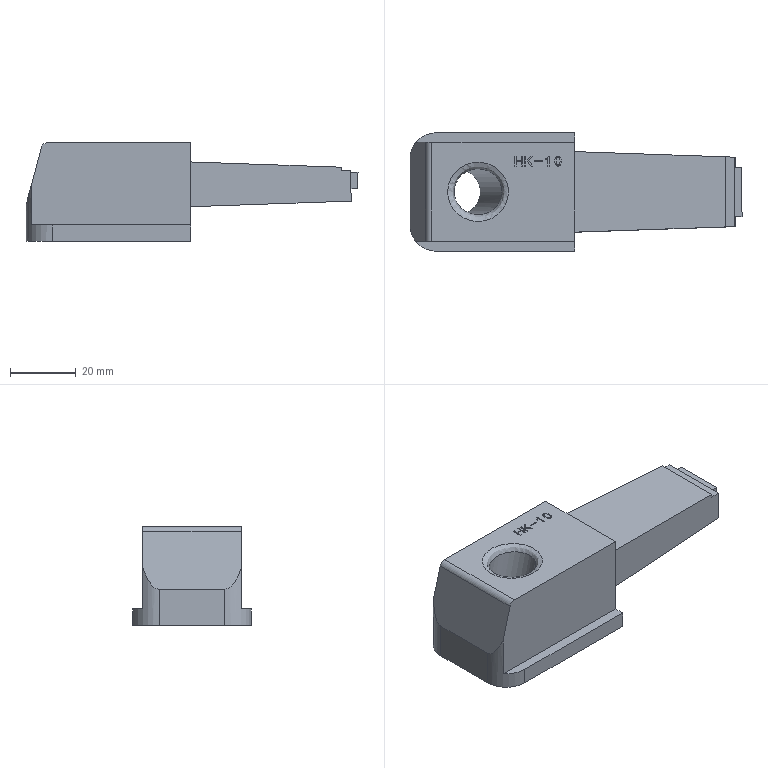Part | STEP file | solid 64 | 1 solid | 76 faces | box 100.766 x 36 x 30 mm | volume 52192 mm3 | plane 63 | other 6 | cylinder 5 | spline 1 | cone 1 | commonest cylinder face diameters 16 x2 4 x1 10 x1 14 x1